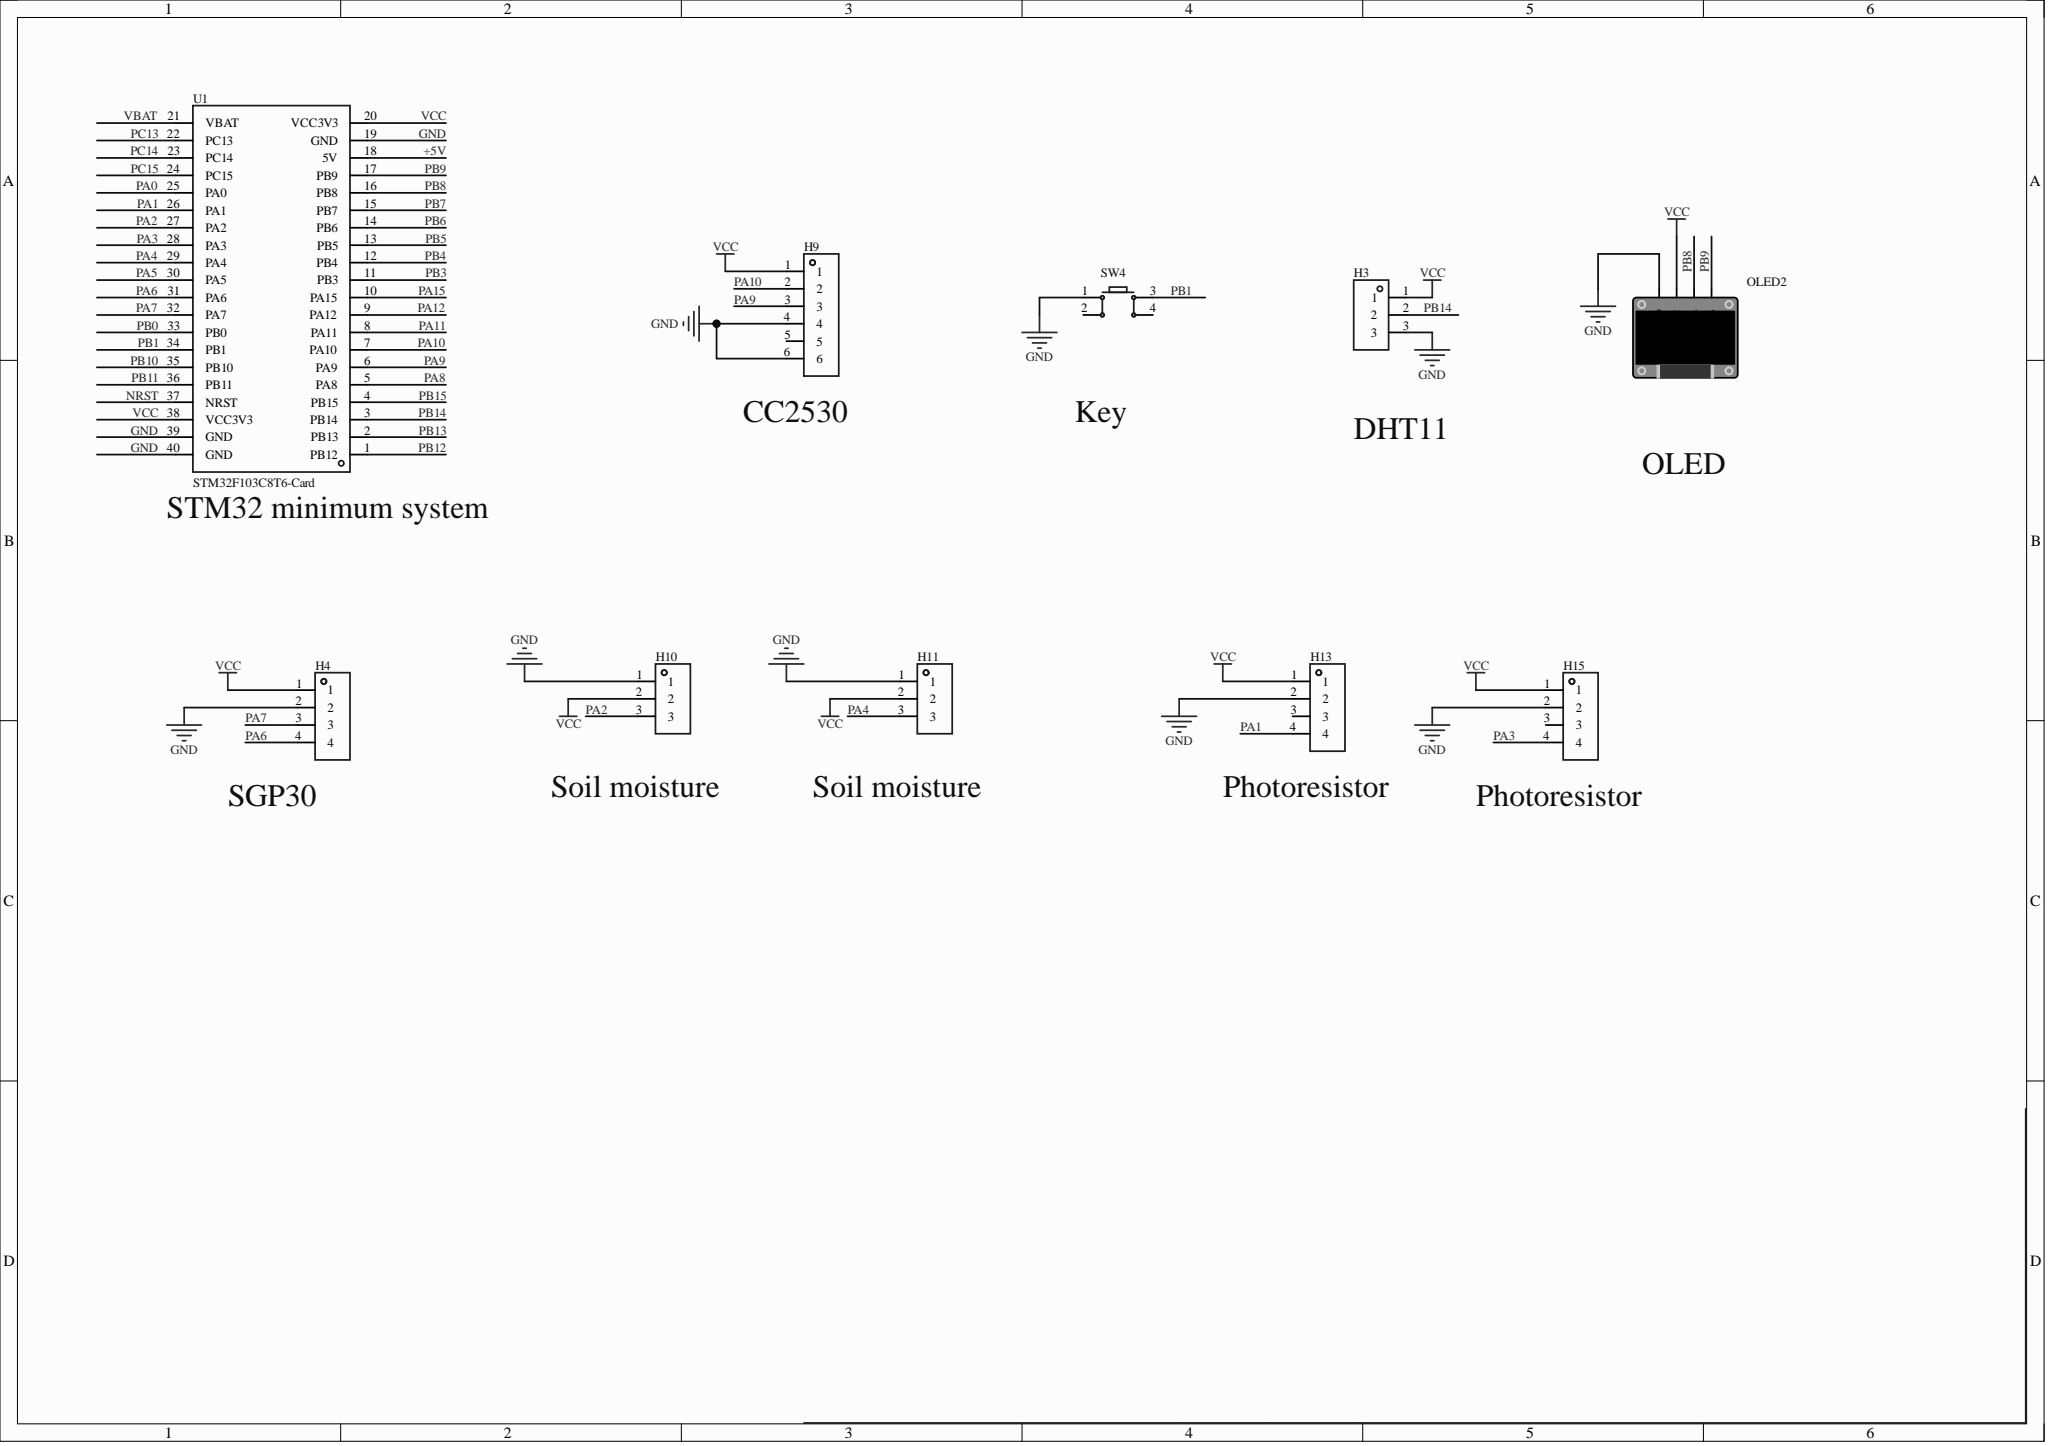Circuit board | Altium Designer | 10 parts | 14 nets
Bill of materials:
Comment,Description,Designator,Footprint,LibRef,Quantity
"","","H3, H10, H11","HDR-TH_3P-P2.54-V-F","HDR-F_2.54_1x3P","3"
"","","H4, H13, H15","HDR-TH_4P-P2.54-V-F","HDR-F_2.54_1x4P","3"
"","","H9","HDR-TH_6P-P2.54-V-F","HDR-F_2.54_1x6P","1"
"","","OLED2","0.96OLED_4P","0.96OLED模块_4P","1"
"","","SW4","SW-TH_4P-L6.0-W6.0-P4.50-LS6.5","Key_TH_6x6x6","1"
"STM32F103C8T6-Card","","U1","CONN-TH_L53.3-W22.9_STM32F103C8T6-CARD","STM32F103C8T6-Card","1"
Netlist (Protel format):
[
H3
HDR-TH_3P-P2.54-V-F




]
[
H4
HDR-TH_4P-P2.54-V-F




]
[
H9
HDR-TH_6P-P2.54-V-F




]
[
H10
HDR-TH_3P-P2.54-V-F




]
[
H11
HDR-TH_3P-P2.54-V-F




]
[
H13
HDR-TH_4P-P2.54-V-F




]
[
H15
HDR-TH_4P-P2.54-V-F




]
[
OLED2
0.96OLED_4P




]
[
SW4
SW-TH_4P-L6.0-W6.0-P4.50-LS6.5




]
[
U1
CONN-TH_L53.3-W22.9_STM32F103C8T6-CARD
STM32F103C8T6-Card



]
(
VCC
H3-1
H4-1
H9-1
H10-2
H11-2
H13-1
H15-1
OLED2-2
U1-20
U1-38
)
(
PB14
H3-2
U1-3
)
(
PB9
OLED2-4
U1-17
)
(
PB8
OLED2-3
U1-16
)
(
PB1
SW4-3
U1-34
)
(
PA10
H9-2
U1-7
)
(
PA9
H9-3
U1-6
)
(
PA7
H4-3
U1-32
)
(
PA6
H4-4
U1-31
)
(
PA4
H11-3
U1-29
)
(
PA3
H15-4
U1-28
)
(
PA2
H10-3
U1-27
)
(
PA1
H13-4
U1-26
)
(
GND
H3-3
H4-2
H9-4
H9-6
H10-1
H11-1
H13-2
H15-2
OLED2-1
SW4-1
U1-19
U1-39
U1-40
)